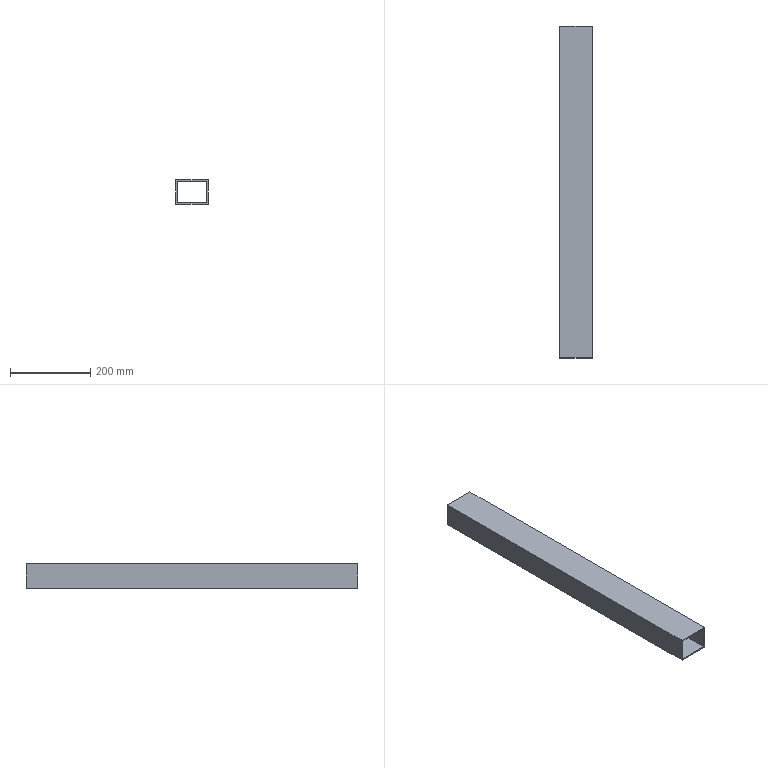Part | STEP file | Guide wheel mechanism revised.sldasm-Part-25 | 1 solid | 10 faces | box 80 x 828.01 x 60 mm | volume 665720 mm3 | plane 10
STEP:
#1=CARTESIAN_POINT('',(405.,828.01,445.));
#2=VERTEX_POINT('',#1);
#3=CARTESIAN_POINT('',(405.,0.,445.));
#4=VERTEX_POINT('',#3);
#5=CARTESIAN_POINT('',(405.,1970.,445.));
#6=DIRECTION('',(0.,-1.,0.));
#7=VECTOR('',#6,1000.);
#8=LINE('',#5,#7);
#9=EDGE_CURVE('',#2,#4,#8,.T.);
#10=ORIENTED_EDGE('',*,*,#9,.F.);
#11=CARTESIAN_POINT('',(485.,828.01,445.));
#12=VERTEX_POINT('',#11);
#13=CARTESIAN_POINT('',(405.,828.01,445.));
#14=DIRECTION('',(-1.,0.,0.));
#15=VECTOR('',#14,1000.);
#16=LINE('',#13,#15);
#17=EDGE_CURVE('',#12,#2,#16,.T.);
#18=ORIENTED_EDGE('',*,*,#17,.F.);
#19=CARTESIAN_POINT('',(485.,0.,445.));
#20=VERTEX_POINT('',#19);
#21=CARTESIAN_POINT('',(485.,1970.,445.));
#22=DIRECTION('',(0.,-1.,0.));
#23=VECTOR('',#22,1000.);
#24=LINE('',#21,#23);
#25=EDGE_CURVE('',#12,#20,#24,.T.);
#26=ORIENTED_EDGE('',*,*,#25,.T.);
#27=CARTESIAN_POINT('',(485.,0.,445.));
#28=DIRECTION('',(-1.,0.,0.));
#29=VECTOR('',#28,1000.);
#30=LINE('',#27,#29);
#31=EDGE_CURVE('',#20,#4,#30,.T.);
#32=ORIENTED_EDGE('',*,*,#31,.T.);
#33=EDGE_LOOP('',(#10,#18,#26,#32));
#34=FACE_OUTER_BOUND('',#33,.T.);
#35=CARTESIAN_POINT('',(485.,1970.,445.));
#36=DIRECTION('',(0.,0.,1.));
#37=DIRECTION('',(1.,0.,0.));
#38=AXIS2_PLACEMENT_3D('',#35,#36,#37);
#39=PLANE('',#38);
#40=ADVANCED_FACE('',(#34),#39,.F.);
#41=ORIENTED_EDGE('',*,*,#25,.F.);
#42=CARTESIAN_POINT('',(485.,828.01,505.));
#43=VERTEX_POINT('',#42);
#44=CARTESIAN_POINT('',(485.,828.01,505.));
#45=DIRECTION('',(0.,0.,1.));
#46=VECTOR('',#45,1000.);
#47=LINE('',#44,#46);
#48=EDGE_CURVE('',#12,#43,#47,.T.);
#49=ORIENTED_EDGE('',*,*,#48,.T.);
#50=CARTESIAN_POINT('',(485.,0.,505.));
#51=VERTEX_POINT('',#50);
#52=CARTESIAN_POINT('',(485.,1970.,505.));
#53=DIRECTION('',(0.,-1.,0.));
#54=VECTOR('',#53,1000.);
#55=LINE('',#52,#54);
#56=EDGE_CURVE('',#43,#51,#55,.T.);
#57=ORIENTED_EDGE('',*,*,#56,.T.);
#58=CARTESIAN_POINT('',(485.,0.,505.));
#59=DIRECTION('',(0.,0.,-1.));
#60=VECTOR('',#59,1000.);
#61=LINE('',#58,#60);
#62=EDGE_CURVE('',#51,#20,#61,.T.);
#63=ORIENTED_EDGE('',*,*,#62,.T.);
#64=EDGE_LOOP('',(#41,#49,#57,#63));
#65=FACE_OUTER_BOUND('',#64,.T.);
#66=CARTESIAN_POINT('',(485.,1970.,505.));
#67=DIRECTION('',(-1.,0.,0.));
#68=DIRECTION('',(0.,0.,1.));
#69=AXIS2_PLACEMENT_3D('',#66,#67,#68);
#70=PLANE('',#69);
#71=ADVANCED_FACE('',(#65),#70,.F.);
#72=ORIENTED_EDGE('',*,*,#56,.F.);
#73=CARTESIAN_POINT('',(405.,828.01,505.));
#74=VERTEX_POINT('',#73);
#75=CARTESIAN_POINT('',(405.,828.01,505.));
#76=DIRECTION('',(1.,0.,0.));
#77=VECTOR('',#76,1000.);
#78=LINE('',#75,#77);
#79=EDGE_CURVE('',#74,#43,#78,.T.);
#80=ORIENTED_EDGE('',*,*,#79,.F.);
#81=CARTESIAN_POINT('',(405.,0.,505.));
#82=VERTEX_POINT('',#81);
#83=CARTESIAN_POINT('',(405.,1970.,505.));
#84=DIRECTION('',(0.,-1.,0.));
#85=VECTOR('',#84,1000.);
#86=LINE('',#83,#85);
#87=EDGE_CURVE('',#74,#82,#86,.T.);
#88=ORIENTED_EDGE('',*,*,#87,.T.);
#89=CARTESIAN_POINT('',(485.,0.,505.));
#90=DIRECTION('',(1.,0.,0.));
#91=VECTOR('',#90,1000.);
#92=LINE('',#89,#91);
#93=EDGE_CURVE('',#82,#51,#92,.T.);
#94=ORIENTED_EDGE('',*,*,#93,.T.);
#95=EDGE_LOOP('',(#72,#80,#88,#94));
#96=FACE_OUTER_BOUND('',#95,.T.);
#97=CARTESIAN_POINT('',(485.,1970.,505.));
#98=DIRECTION('',(0.,0.,-1.));
#99=DIRECTION('',(-1.,0.,0.));
#100=AXIS2_PLACEMENT_3D('',#97,#98,#99);
#101=PLANE('',#100);
#102=ADVANCED_FACE('',(#96),#101,.F.);
#103=ORIENTED_EDGE('',*,*,#87,.F.);
#104=CARTESIAN_POINT('',(405.,828.01,-160.471));
#105=DIRECTION('',(0.,0.,1.));
#106=VECTOR('',#105,1000.);
#107=LINE('',#104,#106);
#108=EDGE_CURVE('',#2,#74,#107,.T.);
#109=ORIENTED_EDGE('',*,*,#108,.F.);
#110=ORIENTED_EDGE('',*,*,#9,.T.);
#111=CARTESIAN_POINT('',(405.,0.,505.));
#112=DIRECTION('',(0.,0.,1.));
#113=VECTOR('',#112,1000.);
#114=LINE('',#111,#113);
#115=EDGE_CURVE('',#4,#82,#114,.T.);
#116=ORIENTED_EDGE('',*,*,#115,.T.);
#117=EDGE_LOOP('',(#103,#109,#110,#116));
#118=FACE_OUTER_BOUND('',#117,.T.);
#119=CARTESIAN_POINT('',(405.,1970.,505.));
#120=DIRECTION('',(1.,0.,0.));
#121=DIRECTION('',(0.,0.,-1.));
#122=AXIS2_PLACEMENT_3D('',#119,#120,#121);
#123=PLANE('',#122);
#124=ADVANCED_FACE('',(#118),#123,.F.);
#125=ORIENTED_EDGE('',*,*,#115,.F.);
#126=ORIENTED_EDGE('',*,*,#31,.F.);
#127=ORIENTED_EDGE('',*,*,#62,.F.);
#128=ORIENTED_EDGE('',*,*,#93,.F.);
#129=EDGE_LOOP('',(#125,#126,#127,#128));
#130=FACE_OUTER_BOUND('',#129,.T.);
#131=CARTESIAN_POINT('',(482.,0.,502.));
#132=VERTEX_POINT('',#131);
#133=CARTESIAN_POINT('',(482.,0.,448.));
#134=VERTEX_POINT('',#133);
#135=CARTESIAN_POINT('',(482.,0.,502.));
#136=DIRECTION('',(0.,0.,-1.));
#137=VECTOR('',#136,1000.);
#138=LINE('',#135,#137);
#139=EDGE_CURVE('',#132,#134,#138,.T.);
#140=ORIENTED_EDGE('',*,*,#139,.T.);
#141=CARTESIAN_POINT('',(408.,0.,448.));
#142=VERTEX_POINT('',#141);
#143=CARTESIAN_POINT('',(482.,0.,448.));
#144=DIRECTION('',(-1.,0.,0.));
#145=VECTOR('',#144,1000.);
#146=LINE('',#143,#145);
#147=EDGE_CURVE('',#134,#142,#146,.T.);
#148=ORIENTED_EDGE('',*,*,#147,.T.);
#149=CARTESIAN_POINT('',(408.,0.,502.));
#150=VERTEX_POINT('',#149);
#151=CARTESIAN_POINT('',(408.,0.,502.));
#152=DIRECTION('',(0.,0.,1.));
#153=VECTOR('',#152,1000.);
#154=LINE('',#151,#153);
#155=EDGE_CURVE('',#142,#150,#154,.T.);
#156=ORIENTED_EDGE('',*,*,#155,.T.);
#157=CARTESIAN_POINT('',(482.,0.,502.));
#158=DIRECTION('',(1.,0.,0.));
#159=VECTOR('',#158,1000.);
#160=LINE('',#157,#159);
#161=EDGE_CURVE('',#150,#132,#160,.T.);
#162=ORIENTED_EDGE('',*,*,#161,.T.);
#163=EDGE_LOOP('',(#140,#148,#156,#162));
#164=FACE_BOUND('',#163,.T.);
#165=CARTESIAN_POINT('',(0.,0.,0.));
#166=DIRECTION('',(0.,1.,0.));
#167=DIRECTION('',(0.,0.,1.));
#168=AXIS2_PLACEMENT_3D('',#165,#166,#167);
#169=PLANE('',#168);
#170=ADVANCED_FACE('',(#130,#164),#169,.F.);
#171=CARTESIAN_POINT('',(482.,828.01,502.));
#172=VERTEX_POINT('',#171);
#173=CARTESIAN_POINT('',(408.,828.01,502.));
#174=VERTEX_POINT('',#173);
#175=CARTESIAN_POINT('',(482.,828.01,502.));
#176=DIRECTION('',(-1.,0.,0.));
#177=VECTOR('',#176,1000.);
#178=LINE('',#175,#177);
#179=EDGE_CURVE('',#172,#174,#178,.T.);
#180=ORIENTED_EDGE('',*,*,#179,.F.);
#181=CARTESIAN_POINT('',(482.,1970.,502.));
#182=DIRECTION('',(0.,-1.,0.));
#183=VECTOR('',#182,1000.);
#184=LINE('',#181,#183);
#185=EDGE_CURVE('',#172,#132,#184,.T.);
#186=ORIENTED_EDGE('',*,*,#185,.T.);
#187=ORIENTED_EDGE('',*,*,#161,.F.);
#188=CARTESIAN_POINT('',(408.,1970.,502.));
#189=DIRECTION('',(0.,-1.,0.));
#190=VECTOR('',#189,1000.);
#191=LINE('',#188,#190);
#192=EDGE_CURVE('',#174,#150,#191,.T.);
#193=ORIENTED_EDGE('',*,*,#192,.F.);
#194=EDGE_LOOP('',(#180,#186,#187,#193));
#195=FACE_OUTER_BOUND('',#194,.T.);
#196=CARTESIAN_POINT('',(482.,1970.,502.));
#197=DIRECTION('',(0.,0.,-1.));
#198=DIRECTION('',(-1.,0.,0.));
#199=AXIS2_PLACEMENT_3D('',#196,#197,#198);
#200=PLANE('',#199);
#201=ADVANCED_FACE('',(#195),#200,.T.);
#202=CARTESIAN_POINT('',(408.,828.01,448.));
#203=VERTEX_POINT('',#202);
#204=CARTESIAN_POINT('',(408.,828.01,502.));
#205=DIRECTION('',(0.,0.,-1.));
#206=VECTOR('',#205,1000.);
#207=LINE('',#204,#206);
#208=EDGE_CURVE('',#174,#203,#207,.T.);
#209=ORIENTED_EDGE('',*,*,#208,.F.);
#210=ORIENTED_EDGE('',*,*,#192,.T.);
#211=ORIENTED_EDGE('',*,*,#155,.F.);
#212=CARTESIAN_POINT('',(408.,1970.,448.));
#213=DIRECTION('',(0.,-1.,0.));
#214=VECTOR('',#213,1000.);
#215=LINE('',#212,#214);
#216=EDGE_CURVE('',#203,#142,#215,.T.);
#217=ORIENTED_EDGE('',*,*,#216,.F.);
#218=EDGE_LOOP('',(#209,#210,#211,#217));
#219=FACE_OUTER_BOUND('',#218,.T.);
#220=CARTESIAN_POINT('',(408.,1970.,502.));
#221=DIRECTION('',(1.,0.,0.));
#222=DIRECTION('',(0.,0.,-1.));
#223=AXIS2_PLACEMENT_3D('',#220,#221,#222);
#224=PLANE('',#223);
#225=ADVANCED_FACE('',(#219),#224,.T.);
#226=CARTESIAN_POINT('',(482.,828.01,448.));
#227=VERTEX_POINT('',#226);
#228=CARTESIAN_POINT('',(482.,828.01,448.));
#229=DIRECTION('',(1.,0.,0.));
#230=VECTOR('',#229,1000.);
#231=LINE('',#228,#230);
#232=EDGE_CURVE('',#203,#227,#231,.T.);
#233=ORIENTED_EDGE('',*,*,#232,.F.);
#234=ORIENTED_EDGE('',*,*,#216,.T.);
#235=ORIENTED_EDGE('',*,*,#147,.F.);
#236=CARTESIAN_POINT('',(482.,1970.,448.));
#237=DIRECTION('',(0.,-1.,0.));
#238=VECTOR('',#237,1000.);
#239=LINE('',#236,#238);
#240=EDGE_CURVE('',#227,#134,#239,.T.);
#241=ORIENTED_EDGE('',*,*,#240,.F.);
#242=EDGE_LOOP('',(#233,#234,#235,#241));
#243=FACE_OUTER_BOUND('',#242,.T.);
#244=CARTESIAN_POINT('',(482.,1970.,448.));
#245=DIRECTION('',(0.,0.,1.));
#246=DIRECTION('',(1.,0.,0.));
#247=AXIS2_PLACEMENT_3D('',#244,#245,#246);
#248=PLANE('',#247);
#249=ADVANCED_FACE('',(#243),#248,.T.);
#250=CARTESIAN_POINT('',(482.,828.01,502.));
#251=DIRECTION('',(0.,0.,1.));
#252=VECTOR('',#251,1000.);
#253=LINE('',#250,#252);
#254=EDGE_CURVE('',#227,#172,#253,.T.);
#255=ORIENTED_EDGE('',*,*,#254,.F.);
#256=ORIENTED_EDGE('',*,*,#240,.T.);
#257=ORIENTED_EDGE('',*,*,#139,.F.);
#258=ORIENTED_EDGE('',*,*,#185,.F.);
#259=EDGE_LOOP('',(#255,#256,#257,#258));
#260=FACE_OUTER_BOUND('',#259,.T.);
#261=CARTESIAN_POINT('',(482.,1970.,502.));
#262=DIRECTION('',(-1.,0.,0.));
#263=DIRECTION('',(0.,0.,1.));
#264=AXIS2_PLACEMENT_3D('',#261,#262,#263);
#265=PLANE('',#264);
#266=ADVANCED_FACE('',(#260),#265,.T.);
#267=ORIENTED_EDGE('',*,*,#254,.T.);
#268=ORIENTED_EDGE('',*,*,#179,.T.);
#269=ORIENTED_EDGE('',*,*,#208,.T.);
#270=ORIENTED_EDGE('',*,*,#232,.T.);
#271=EDGE_LOOP('',(#267,#268,#269,#270));
#272=FACE_BOUND('',#271,.T.);
#273=ORIENTED_EDGE('',*,*,#17,.T.);
#274=ORIENTED_EDGE('',*,*,#108,.T.);
#275=ORIENTED_EDGE('',*,*,#79,.T.);
#276=ORIENTED_EDGE('',*,*,#48,.F.);
#277=EDGE_LOOP('',(#273,#274,#275,#276));
#278=FACE_OUTER_BOUND('',#277,.T.);
#279=CARTESIAN_POINT('',(405.,828.01,-160.471));
#280=DIRECTION('',(0.,-1.,0.));
#281=DIRECTION('',(0.,0.,-1.));
#282=AXIS2_PLACEMENT_3D('',#279,#280,#281);
#283=PLANE('',#282);
#284=ADVANCED_FACE('',(#272,#278),#283,.F.);
#285=CLOSED_SHELL('',(#40,#71,#102,#124,#170,#201,#225,#249,#266,#284));
#286=MANIFOLD_SOLID_BREP('',#285);
#287=CARTESIAN_POINT('',(0.,0.,0.));
#288=DIRECTION('',(0.,0.,1.));
#289=DIRECTION('',(1.,0.,0.));
#290=AXIS2_PLACEMENT_3D('',#287,#288,#289);
#291=(LENGTH_UNIT()NAMED_UNIT(*)SI_UNIT(.MILLI.,.METRE.));
#292=UNCERTAINTY_MEASURE_WITH_UNIT(LENGTH_MEASURE(0.00001),#291,'','');
#293=(NAMED_UNIT(*)PLANE_ANGLE_UNIT()SI_UNIT($,.RADIAN.));
#294=(NAMED_UNIT(*)SI_UNIT($,.STERADIAN.)SOLID_ANGLE_UNIT());
#295=(GEOMETRIC_REPRESENTATION_CONTEXT(3)GLOBAL_UNCERTAINTY_ASSIGNED_CONTEXT((#292))GLOBAL_UNIT_ASSIGNED_CONTEXT((#291,#293,#294))REPRESENTATION_CONTEXT('',''));
#296=ADVANCED_BREP_SHAPE_REPRESENTATION('',(#286,#290),#295);